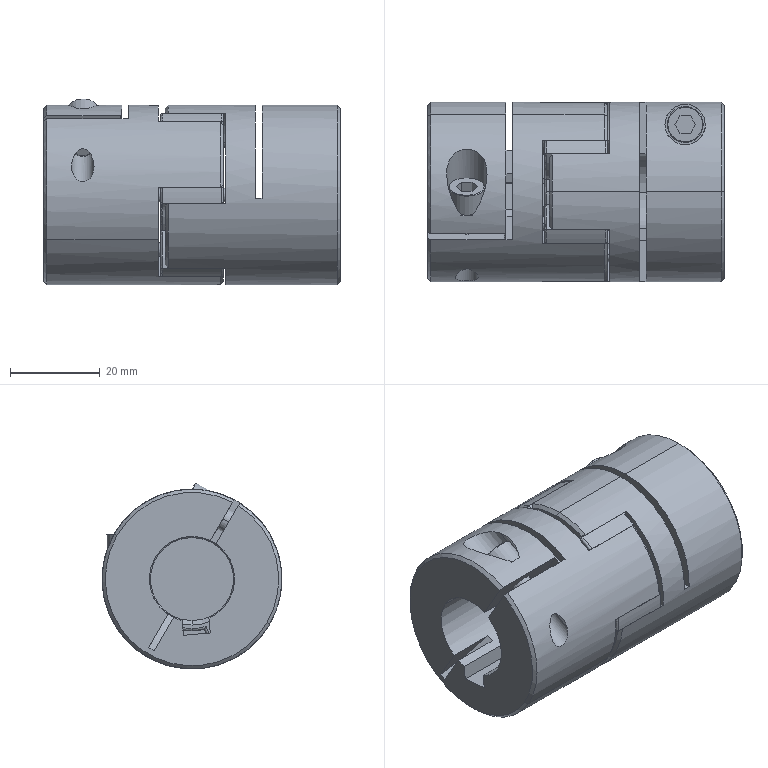Part | STEP file | coupling DEP12-D40L-d17-e19-DC-DD | 5 solids | 245 faces | box 66 x 40 x 41.384 mm | volume 61965 mm3 | cylinder 98 | plane 67 | torus 54 | cone 26 | commonest cylinder face diameters 23 x33 3 x12 40 x10 5 x8 24 x8 9 x6